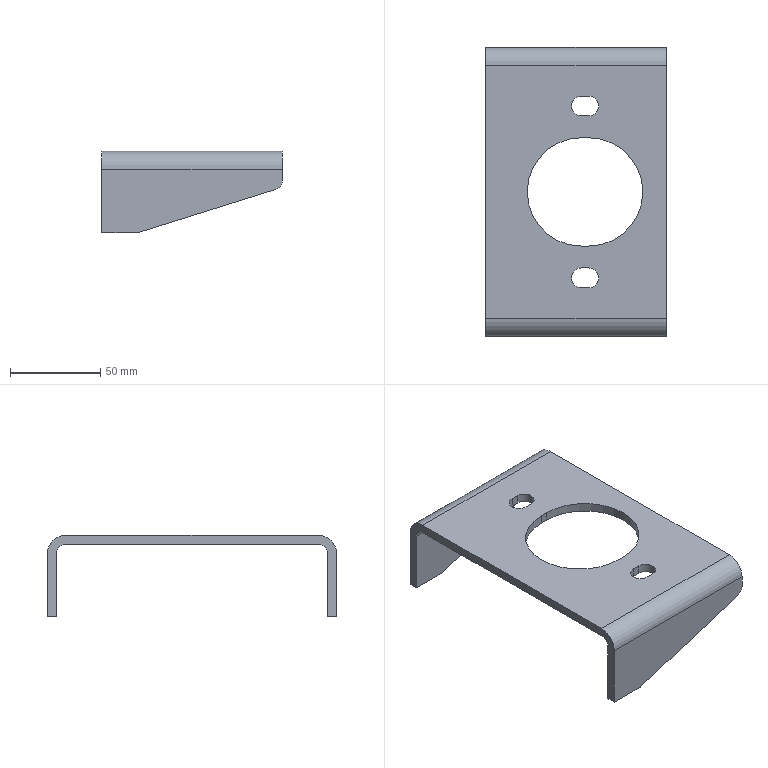Part | STEP file | HL4GD-1.30.107 cab vibration-damping mounting bracket-
-20251212 | 1 solid | 32 faces | box 100 x 160 x 45 mm | volume 90028 mm3 | plane 18 | cylinder 14 | commonest cylinder face diameters 10 x6 11 x4 20 x2 60 x2